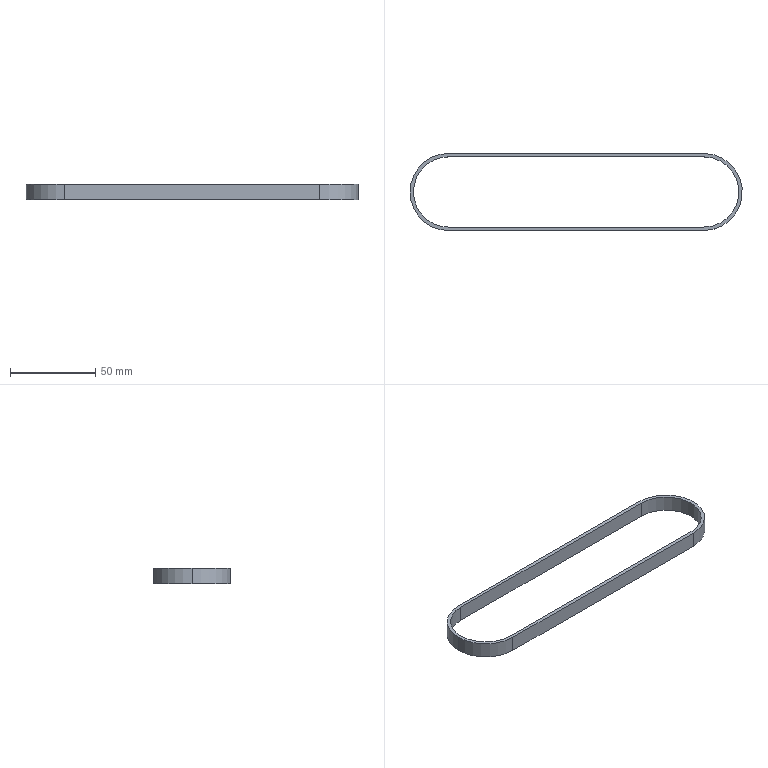Part | SolidWorks | features ExtruThin 1 | 1 solid | 12 faces | box 195.3 x 45.3 x 9.4 mm | volume 8197 mm3 | cylinder 6 | plane 6 | commonest cylinder face diameters 41.3 x3 45.3 x3
STEP:
#1=CARTESIAN_POINT('',(0.,20.65,4.7));
#2=VERTEX_POINT('',#1);
#3=CARTESIAN_POINT('',(-20.65,0.,4.7));
#4=VERTEX_POINT('',#3);
#5=CARTESIAN_POINT('',(0.,0.,4.7));
#6=DIRECTION('',(0.,0.,1.));
#7=DIRECTION('',(1.,0.,0.));
#8=AXIS2_PLACEMENT_3D('',#5,#6,#7);
#9=CIRCLE('',#8,20.65);
#10=EDGE_CURVE('',#2,#4,#9,.T.);
#11=ORIENTED_EDGE('',*,*,#10,.T.);
#12=CARTESIAN_POINT('',(-20.65,0.,-4.7));
#13=VERTEX_POINT('',#12);
#14=CARTESIAN_POINT('',(-20.65,0.,4.7));
#15=DIRECTION('',(0.,0.,-1.));
#16=VECTOR('',#15,1000.);
#17=LINE('',#14,#16);
#18=EDGE_CURVE('',#4,#13,#17,.T.);
#19=ORIENTED_EDGE('',*,*,#18,.T.);
#20=CARTESIAN_POINT('',(0.,20.65,-4.7));
#21=VERTEX_POINT('',#20);
#22=CARTESIAN_POINT('',(0.,0.,-4.7));
#23=DIRECTION('',(0.,0.,1.));
#24=DIRECTION('',(1.,0.,0.));
#25=AXIS2_PLACEMENT_3D('',#22,#23,#24);
#26=CIRCLE('',#25,20.65);
#27=EDGE_CURVE('',#21,#13,#26,.T.);
#28=ORIENTED_EDGE('',*,*,#27,.F.);
#29=CARTESIAN_POINT('',(0.,20.65,4.7));
#30=DIRECTION('',(0.,0.,-1.));
#31=VECTOR('',#30,1000.);
#32=LINE('',#29,#31);
#33=EDGE_CURVE('',#2,#21,#32,.T.);
#34=ORIENTED_EDGE('',*,*,#33,.F.);
#35=EDGE_LOOP('',(#11,#19,#28,#34));
#36=FACE_OUTER_BOUND('',#35,.T.);
#37=CARTESIAN_POINT('',(0.,0.,4.7));
#38=DIRECTION('',(0.,0.,-1.));
#39=DIRECTION('',(-1.,0.,0.));
#40=AXIS2_PLACEMENT_3D('',#37,#38,#39);
#41=CYLINDRICAL_SURFACE('',#40,20.65);
#42=ADVANCED_FACE('',(#36),#41,.F.);
#43=CARTESIAN_POINT('',(-22.65,0.,4.7));
#44=VERTEX_POINT('',#43);
#45=CARTESIAN_POINT('',(0.,-22.65,4.7));
#46=VERTEX_POINT('',#45);
#47=CARTESIAN_POINT('',(0.,0.,4.7));
#48=DIRECTION('',(0.,0.,1.));
#49=DIRECTION('',(1.,0.,0.));
#50=AXIS2_PLACEMENT_3D('',#47,#48,#49);
#51=CIRCLE('',#50,22.65);
#52=EDGE_CURVE('',#44,#46,#51,.T.);
#53=ORIENTED_EDGE('',*,*,#52,.F.);
#54=CARTESIAN_POINT('',(-22.65,0.,-4.7));
#55=VERTEX_POINT('',#54);
#56=CARTESIAN_POINT('',(-22.65,0.,4.7));
#57=DIRECTION('',(0.,0.,-1.));
#58=VECTOR('',#57,1000.);
#59=LINE('',#56,#58);
#60=EDGE_CURVE('',#44,#55,#59,.T.);
#61=ORIENTED_EDGE('',*,*,#60,.T.);
#62=CARTESIAN_POINT('',(0.,-22.65,-4.7));
#63=VERTEX_POINT('',#62);
#64=CARTESIAN_POINT('',(0.,0.,-4.7));
#65=DIRECTION('',(0.,0.,1.));
#66=DIRECTION('',(1.,0.,0.));
#67=AXIS2_PLACEMENT_3D('',#64,#65,#66);
#68=CIRCLE('',#67,22.65);
#69=EDGE_CURVE('',#55,#63,#68,.T.);
#70=ORIENTED_EDGE('',*,*,#69,.T.);
#71=CARTESIAN_POINT('',(0.,-22.65,4.7));
#72=DIRECTION('',(0.,0.,-1.));
#73=VECTOR('',#72,1000.);
#74=LINE('',#71,#73);
#75=EDGE_CURVE('',#46,#63,#74,.T.);
#76=ORIENTED_EDGE('',*,*,#75,.F.);
#77=EDGE_LOOP('',(#53,#61,#70,#76));
#78=FACE_OUTER_BOUND('',#77,.T.);
#79=CARTESIAN_POINT('',(0.,0.,4.7));
#80=DIRECTION('',(0.,0.,-1.));
#81=DIRECTION('',(-1.,0.,0.));
#82=AXIS2_PLACEMENT_3D('',#79,#80,#81);
#83=CYLINDRICAL_SURFACE('',#82,22.65);
#84=ADVANCED_FACE('',(#78),#83,.T.);
#85=CARTESIAN_POINT('',(0.,22.65,4.7));
#86=VERTEX_POINT('',#85);
#87=CARTESIAN_POINT('',(0.,0.,4.7));
#88=DIRECTION('',(0.,0.,1.));
#89=DIRECTION('',(1.,0.,0.));
#90=AXIS2_PLACEMENT_3D('',#87,#88,#89);
#91=CIRCLE('',#90,22.65);
#92=EDGE_CURVE('',#86,#44,#91,.T.);
#93=ORIENTED_EDGE('',*,*,#92,.T.);
#94=ORIENTED_EDGE('',*,*,#52,.T.);
#95=CARTESIAN_POINT('',(150.,-22.65,4.7));
#96=VERTEX_POINT('',#95);
#97=CARTESIAN_POINT('',(0.,-22.65,4.7));
#98=DIRECTION('',(1.,0.,0.));
#99=VECTOR('',#98,1000.);
#100=LINE('',#97,#99);
#101=EDGE_CURVE('',#46,#96,#100,.T.);
#102=ORIENTED_EDGE('',*,*,#101,.T.);
#103=CARTESIAN_POINT('',(150.,22.65,4.7));
#104=VERTEX_POINT('',#103);
#105=CARTESIAN_POINT('',(150.,0.,4.7));
#106=DIRECTION('',(0.,0.,1.));
#107=DIRECTION('',(1.,0.,0.));
#108=AXIS2_PLACEMENT_3D('',#105,#106,#107);
#109=CIRCLE('',#108,22.65);
#110=EDGE_CURVE('',#96,#104,#109,.T.);
#111=ORIENTED_EDGE('',*,*,#110,.T.);
#112=CARTESIAN_POINT('',(0.,22.65,4.7));
#113=DIRECTION('',(-1.,0.,0.));
#114=VECTOR('',#113,1000.);
#115=LINE('',#112,#114);
#116=EDGE_CURVE('',#104,#86,#115,.T.);
#117=ORIENTED_EDGE('',*,*,#116,.T.);
#118=EDGE_LOOP('',(#93,#94,#102,#111,#117));
#119=FACE_OUTER_BOUND('',#118,.T.);
#120=CARTESIAN_POINT('',(0.,-20.65,4.7));
#121=VERTEX_POINT('',#120);
#122=CARTESIAN_POINT('',(150.,-20.65,4.7));
#123=VERTEX_POINT('',#122);
#124=CARTESIAN_POINT('',(0.,-20.65,4.7));
#125=DIRECTION('',(1.,0.,0.));
#126=VECTOR('',#125,1000.);
#127=LINE('',#124,#126);
#128=EDGE_CURVE('',#121,#123,#127,.T.);
#129=ORIENTED_EDGE('',*,*,#128,.F.);
#130=CARTESIAN_POINT('',(0.,0.,4.7));
#131=DIRECTION('',(0.,0.,1.));
#132=DIRECTION('',(1.,0.,0.));
#133=AXIS2_PLACEMENT_3D('',#130,#131,#132);
#134=CIRCLE('',#133,20.65);
#135=EDGE_CURVE('',#4,#121,#134,.T.);
#136=ORIENTED_EDGE('',*,*,#135,.F.);
#137=ORIENTED_EDGE('',*,*,#10,.F.);
#138=CARTESIAN_POINT('',(150.,20.65,4.7));
#139=VERTEX_POINT('',#138);
#140=CARTESIAN_POINT('',(0.,20.65,4.7));
#141=DIRECTION('',(-1.,0.,0.));
#142=VECTOR('',#141,1000.);
#143=LINE('',#140,#142);
#144=EDGE_CURVE('',#139,#2,#143,.T.);
#145=ORIENTED_EDGE('',*,*,#144,.F.);
#146=CARTESIAN_POINT('',(150.,0.,4.7));
#147=DIRECTION('',(0.,0.,1.));
#148=DIRECTION('',(1.,0.,0.));
#149=AXIS2_PLACEMENT_3D('',#146,#147,#148);
#150=CIRCLE('',#149,20.65);
#151=EDGE_CURVE('',#123,#139,#150,.T.);
#152=ORIENTED_EDGE('',*,*,#151,.F.);
#153=EDGE_LOOP('',(#129,#136,#137,#145,#152));
#154=FACE_BOUND('',#153,.T.);
#155=CARTESIAN_POINT('',(0.,0.,4.7));
#156=DIRECTION('',(0.,0.,1.));
#157=DIRECTION('',(1.,0.,0.));
#158=AXIS2_PLACEMENT_3D('',#155,#156,#157);
#159=PLANE('',#158);
#160=ADVANCED_FACE('',(#119,#154),#159,.T.);
#161=CARTESIAN_POINT('',(0.,22.65,-4.7));
#162=VERTEX_POINT('',#161);
#163=CARTESIAN_POINT('',(0.,0.,-4.7));
#164=DIRECTION('',(0.,0.,1.));
#165=DIRECTION('',(1.,0.,0.));
#166=AXIS2_PLACEMENT_3D('',#163,#164,#165);
#167=CIRCLE('',#166,22.65);
#168=EDGE_CURVE('',#162,#55,#167,.T.);
#169=ORIENTED_EDGE('',*,*,#168,.F.);
#170=CARTESIAN_POINT('',(150.,22.65,-4.7));
#171=VERTEX_POINT('',#170);
#172=CARTESIAN_POINT('',(0.,22.65,-4.7));
#173=DIRECTION('',(-1.,0.,0.));
#174=VECTOR('',#173,1000.);
#175=LINE('',#172,#174);
#176=EDGE_CURVE('',#171,#162,#175,.T.);
#177=ORIENTED_EDGE('',*,*,#176,.F.);
#178=CARTESIAN_POINT('',(150.,-22.65,-4.7));
#179=VERTEX_POINT('',#178);
#180=CARTESIAN_POINT('',(150.,0.,-4.7));
#181=DIRECTION('',(0.,0.,1.));
#182=DIRECTION('',(1.,0.,0.));
#183=AXIS2_PLACEMENT_3D('',#180,#181,#182);
#184=CIRCLE('',#183,22.65);
#185=EDGE_CURVE('',#179,#171,#184,.T.);
#186=ORIENTED_EDGE('',*,*,#185,.F.);
#187=CARTESIAN_POINT('',(0.,-22.65,-4.7));
#188=DIRECTION('',(1.,0.,0.));
#189=VECTOR('',#188,1000.);
#190=LINE('',#187,#189);
#191=EDGE_CURVE('',#63,#179,#190,.T.);
#192=ORIENTED_EDGE('',*,*,#191,.F.);
#193=ORIENTED_EDGE('',*,*,#69,.F.);
#194=EDGE_LOOP('',(#169,#177,#186,#192,#193));
#195=FACE_OUTER_BOUND('',#194,.T.);
#196=ORIENTED_EDGE('',*,*,#27,.T.);
#197=CARTESIAN_POINT('',(0.,-20.65,-4.7));
#198=VERTEX_POINT('',#197);
#199=CARTESIAN_POINT('',(0.,0.,-4.7));
#200=DIRECTION('',(0.,0.,1.));
#201=DIRECTION('',(1.,0.,0.));
#202=AXIS2_PLACEMENT_3D('',#199,#200,#201);
#203=CIRCLE('',#202,20.65);
#204=EDGE_CURVE('',#13,#198,#203,.T.);
#205=ORIENTED_EDGE('',*,*,#204,.T.);
#206=CARTESIAN_POINT('',(150.,-20.65,-4.7));
#207=VERTEX_POINT('',#206);
#208=CARTESIAN_POINT('',(0.,-20.65,-4.7));
#209=DIRECTION('',(1.,0.,0.));
#210=VECTOR('',#209,1000.);
#211=LINE('',#208,#210);
#212=EDGE_CURVE('',#198,#207,#211,.T.);
#213=ORIENTED_EDGE('',*,*,#212,.T.);
#214=CARTESIAN_POINT('',(150.,20.65,-4.7));
#215=VERTEX_POINT('',#214);
#216=CARTESIAN_POINT('',(150.,0.,-4.7));
#217=DIRECTION('',(0.,0.,1.));
#218=DIRECTION('',(1.,0.,0.));
#219=AXIS2_PLACEMENT_3D('',#216,#217,#218);
#220=CIRCLE('',#219,20.65);
#221=EDGE_CURVE('',#207,#215,#220,.T.);
#222=ORIENTED_EDGE('',*,*,#221,.T.);
#223=CARTESIAN_POINT('',(0.,20.65,-4.7));
#224=DIRECTION('',(-1.,0.,0.));
#225=VECTOR('',#224,1000.);
#226=LINE('',#223,#225);
#227=EDGE_CURVE('',#215,#21,#226,.T.);
#228=ORIENTED_EDGE('',*,*,#227,.T.);
#229=EDGE_LOOP('',(#196,#205,#213,#222,#228));
#230=FACE_BOUND('',#229,.T.);
#231=CARTESIAN_POINT('',(0.,0.,-4.7));
#232=DIRECTION('',(0.,0.,1.));
#233=DIRECTION('',(1.,0.,0.));
#234=AXIS2_PLACEMENT_3D('',#231,#232,#233);
#235=PLANE('',#234);
#236=ADVANCED_FACE('',(#195,#230),#235,.F.);
#237=ORIENTED_EDGE('',*,*,#60,.F.);
#238=ORIENTED_EDGE('',*,*,#92,.F.);
#239=CARTESIAN_POINT('',(0.,22.65,4.7));
#240=DIRECTION('',(0.,0.,-1.));
#241=VECTOR('',#240,1000.);
#242=LINE('',#239,#241);
#243=EDGE_CURVE('',#86,#162,#242,.T.);
#244=ORIENTED_EDGE('',*,*,#243,.T.);
#245=ORIENTED_EDGE('',*,*,#168,.T.);
#246=EDGE_LOOP('',(#237,#238,#244,#245));
#247=FACE_OUTER_BOUND('',#246,.T.);
#248=CARTESIAN_POINT('',(0.,0.,4.7));
#249=DIRECTION('',(0.,0.,-1.));
#250=DIRECTION('',(-1.,0.,0.));
#251=AXIS2_PLACEMENT_3D('',#248,#249,#250);
#252=CYLINDRICAL_SURFACE('',#251,22.65);
#253=ADVANCED_FACE('',(#247),#252,.T.);
#254=ORIENTED_EDGE('',*,*,#191,.T.);
#255=CARTESIAN_POINT('',(150.,-22.65,4.7));
#256=DIRECTION('',(0.,0.,-1.));
#257=VECTOR('',#256,1000.);
#258=LINE('',#255,#257);
#259=EDGE_CURVE('',#96,#179,#258,.T.);
#260=ORIENTED_EDGE('',*,*,#259,.F.);
#261=ORIENTED_EDGE('',*,*,#101,.F.);
#262=ORIENTED_EDGE('',*,*,#75,.T.);
#263=EDGE_LOOP('',(#254,#260,#261,#262));
#264=FACE_OUTER_BOUND('',#263,.T.);
#265=CARTESIAN_POINT('',(0.,-22.65,4.7));
#266=DIRECTION('',(0.,1.,0.));
#267=DIRECTION('',(0.,0.,1.));
#268=AXIS2_PLACEMENT_3D('',#265,#266,#267);
#269=PLANE('',#268);
#270=ADVANCED_FACE('',(#264),#269,.F.);
#271=ORIENTED_EDGE('',*,*,#185,.T.);
#272=CARTESIAN_POINT('',(150.,22.65,4.7));
#273=DIRECTION('',(0.,0.,-1.));
#274=VECTOR('',#273,1000.);
#275=LINE('',#272,#274);
#276=EDGE_CURVE('',#104,#171,#275,.T.);
#277=ORIENTED_EDGE('',*,*,#276,.F.);
#278=ORIENTED_EDGE('',*,*,#110,.F.);
#279=ORIENTED_EDGE('',*,*,#259,.T.);
#280=EDGE_LOOP('',(#271,#277,#278,#279));
#281=FACE_OUTER_BOUND('',#280,.T.);
#282=CARTESIAN_POINT('',(150.,0.,4.7));
#283=DIRECTION('',(0.,0.,-1.));
#284=DIRECTION('',(-1.,0.,0.));
#285=AXIS2_PLACEMENT_3D('',#282,#283,#284);
#286=CYLINDRICAL_SURFACE('',#285,22.65);
#287=ADVANCED_FACE('',(#281),#286,.T.);
#288=ORIENTED_EDGE('',*,*,#176,.T.);
#289=ORIENTED_EDGE('',*,*,#243,.F.);
#290=ORIENTED_EDGE('',*,*,#116,.F.);
#291=ORIENTED_EDGE('',*,*,#276,.T.);
#292=EDGE_LOOP('',(#288,#289,#290,#291));
#293=FACE_OUTER_BOUND('',#292,.T.);
#294=CARTESIAN_POINT('',(0.,22.65,4.7));
#295=DIRECTION('',(0.,-1.,0.));
#296=DIRECTION('',(0.,0.,-1.));
#297=AXIS2_PLACEMENT_3D('',#294,#295,#296);
#298=PLANE('',#297);
#299=ADVANCED_FACE('',(#293),#298,.F.);
#300=ORIENTED_EDGE('',*,*,#18,.F.);
#301=ORIENTED_EDGE('',*,*,#135,.T.);
#302=CARTESIAN_POINT('',(0.,-20.65,4.7));
#303=DIRECTION('',(0.,0.,-1.));
#304=VECTOR('',#303,1000.);
#305=LINE('',#302,#304);
#306=EDGE_CURVE('',#121,#198,#305,.T.);
#307=ORIENTED_EDGE('',*,*,#306,.T.);
#308=ORIENTED_EDGE('',*,*,#204,.F.);
#309=EDGE_LOOP('',(#300,#301,#307,#308));
#310=FACE_OUTER_BOUND('',#309,.T.);
#311=CARTESIAN_POINT('',(0.,0.,4.7));
#312=DIRECTION('',(0.,0.,-1.));
#313=DIRECTION('',(-1.,0.,0.));
#314=AXIS2_PLACEMENT_3D('',#311,#312,#313);
#315=CYLINDRICAL_SURFACE('',#314,20.65);
#316=ADVANCED_FACE('',(#310),#315,.F.);
#317=ORIENTED_EDGE('',*,*,#212,.F.);
#318=ORIENTED_EDGE('',*,*,#306,.F.);
#319=ORIENTED_EDGE('',*,*,#128,.T.);
#320=CARTESIAN_POINT('',(150.,-20.65,4.7));
#321=DIRECTION('',(0.,0.,-1.));
#322=VECTOR('',#321,1000.);
#323=LINE('',#320,#322);
#324=EDGE_CURVE('',#123,#207,#323,.T.);
#325=ORIENTED_EDGE('',*,*,#324,.T.);
#326=EDGE_LOOP('',(#317,#318,#319,#325));
#327=FACE_OUTER_BOUND('',#326,.T.);
#328=CARTESIAN_POINT('',(0.,-20.65,4.7));
#329=DIRECTION('',(0.,1.,0.));
#330=DIRECTION('',(0.,0.,1.));
#331=AXIS2_PLACEMENT_3D('',#328,#329,#330);
#332=PLANE('',#331);
#333=ADVANCED_FACE('',(#327),#332,.T.);
#334=ORIENTED_EDGE('',*,*,#221,.F.);
#335=ORIENTED_EDGE('',*,*,#324,.F.);
#336=ORIENTED_EDGE('',*,*,#151,.T.);
#337=CARTESIAN_POINT('',(150.,20.65,4.7));
#338=DIRECTION('',(0.,0.,-1.));
#339=VECTOR('',#338,1000.);
#340=LINE('',#337,#339);
#341=EDGE_CURVE('',#139,#215,#340,.T.);
#342=ORIENTED_EDGE('',*,*,#341,.T.);
#343=EDGE_LOOP('',(#334,#335,#336,#342));
#344=FACE_OUTER_BOUND('',#343,.T.);
#345=CARTESIAN_POINT('',(150.,0.,4.7));
#346=DIRECTION('',(0.,0.,-1.));
#347=DIRECTION('',(-1.,0.,0.));
#348=AXIS2_PLACEMENT_3D('',#345,#346,#347);
#349=CYLINDRICAL_SURFACE('',#348,20.65);
#350=ADVANCED_FACE('',(#344),#349,.F.);
#351=ORIENTED_EDGE('',*,*,#227,.F.);
#352=ORIENTED_EDGE('',*,*,#341,.F.);
#353=ORIENTED_EDGE('',*,*,#144,.T.);
#354=ORIENTED_EDGE('',*,*,#33,.T.);
#355=EDGE_LOOP('',(#351,#352,#353,#354));
#356=FACE_OUTER_BOUND('',#355,.T.);
#357=CARTESIAN_POINT('',(0.,20.65,4.7));
#358=DIRECTION('',(0.,-1.,0.));
#359=DIRECTION('',(0.,0.,-1.));
#360=AXIS2_PLACEMENT_3D('',#357,#358,#359);
#361=PLANE('',#360);
#362=ADVANCED_FACE('',(#356),#361,.T.);
#363=CLOSED_SHELL('',(#42,#84,#160,#236,#253,#270,#287,#299,#316,#333,#350,#362));
#364=MANIFOLD_SOLID_BREP('',#363);
#365=CARTESIAN_POINT('',(0.,0.,0.));
#366=DIRECTION('',(0.,0.,1.));
#367=DIRECTION('',(1.,0.,0.));
#368=AXIS2_PLACEMENT_3D('',#365,#366,#367);
#369=(LENGTH_UNIT()NAMED_UNIT(*)SI_UNIT(.MILLI.,.METRE.));
#370=UNCERTAINTY_MEASURE_WITH_UNIT(LENGTH_MEASURE(0.00001),#369,'','');
#371=(NAMED_UNIT(*)PLANE_ANGLE_UNIT()SI_UNIT($,.RADIAN.));
#372=(NAMED_UNIT(*)SI_UNIT($,.STERADIAN.)SOLID_ANGLE_UNIT());
#373=(GEOMETRIC_REPRESENTATION_CONTEXT(3)GLOBAL_UNCERTAINTY_ASSIGNED_CONTEXT((#370))GLOBAL_UNIT_ASSIGNED_CONTEXT((#369,#371,#372))REPRESENTATION_CONTEXT('',''));
#374=ADVANCED_BREP_SHAPE_REPRESENTATION('',(#364,#368),#373);